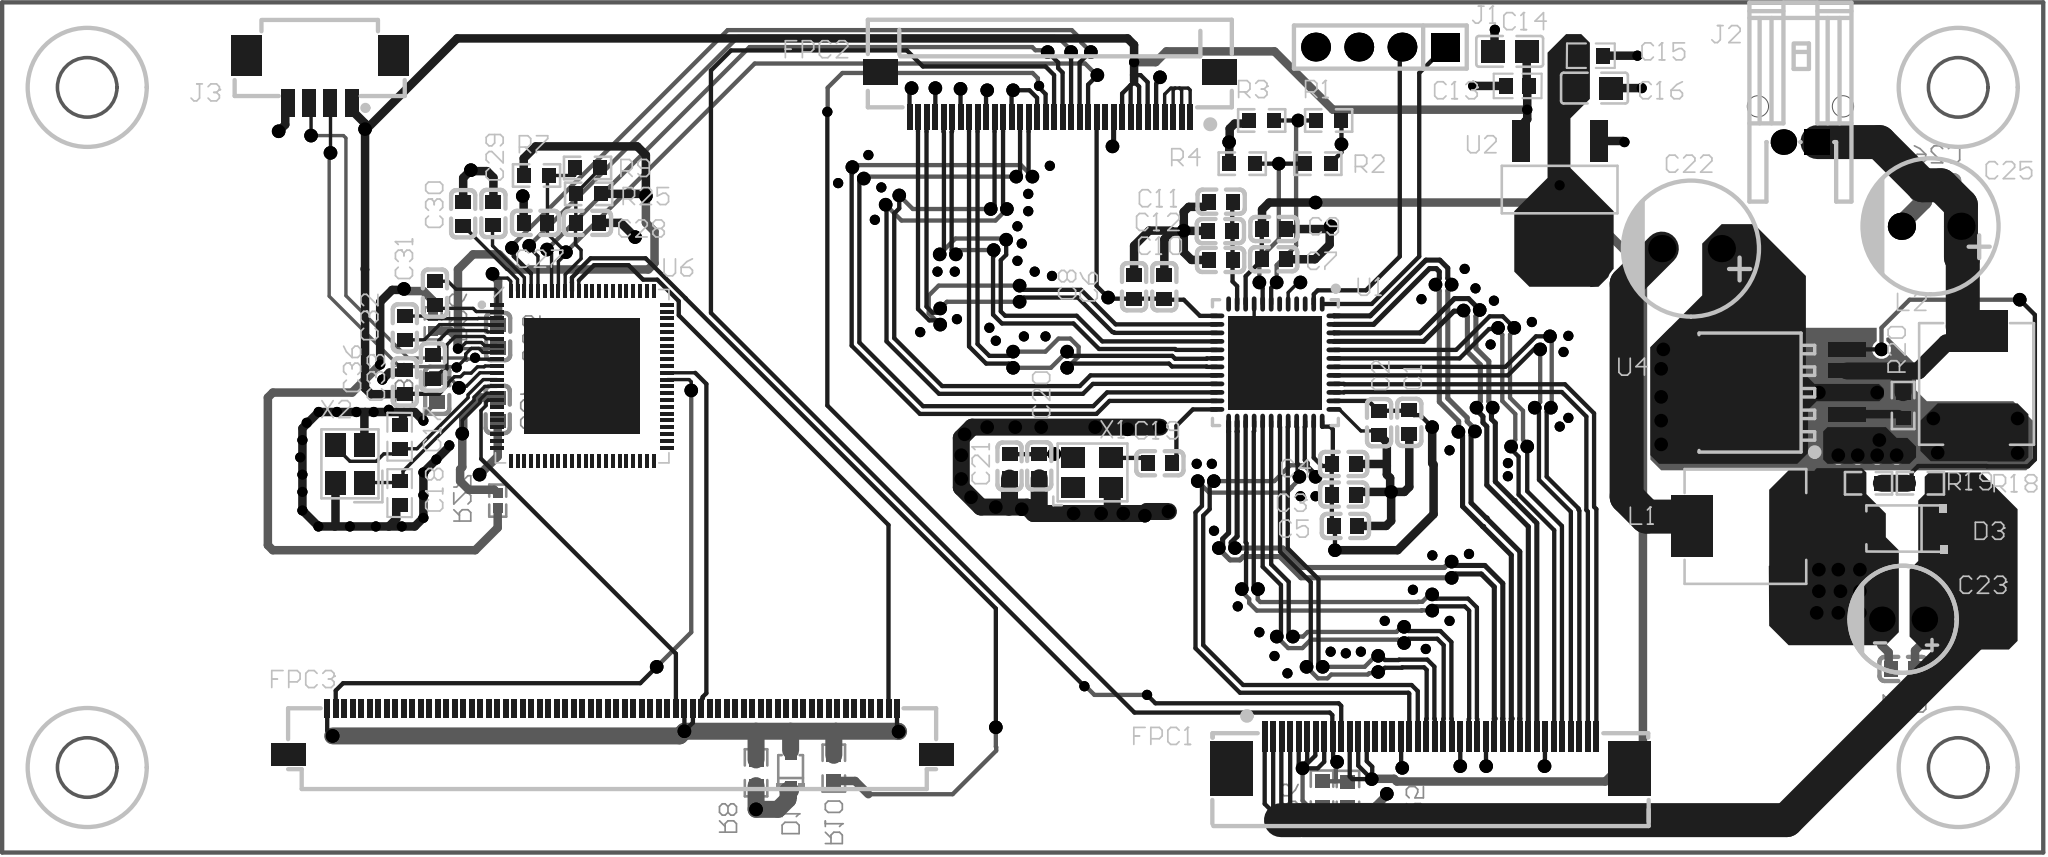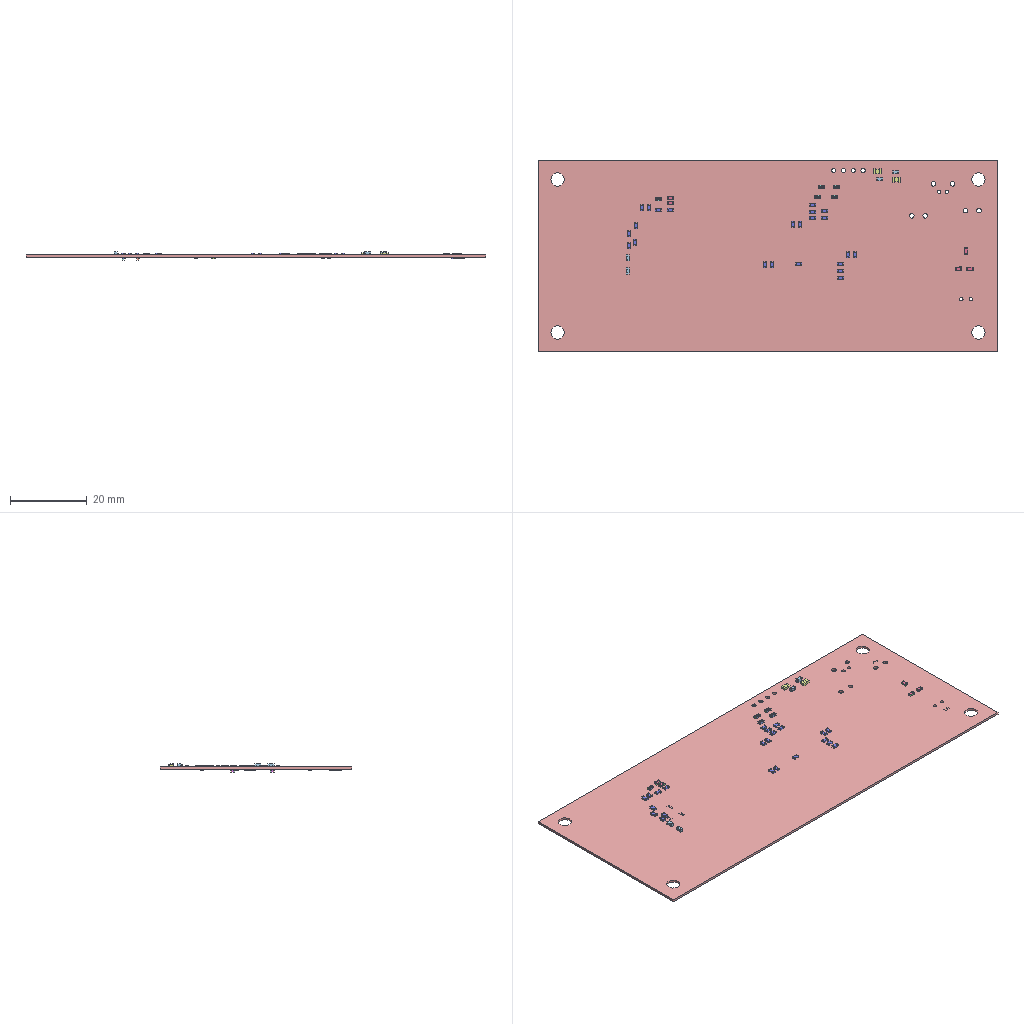Circuit board layout | Altium Designer | box 120 x 50 x 2.1 mm
Part placement:
Designator,Comment,Layer,Footprint,Center-X(mm),Center-Y(mm),Rotation
R10,0R 0603,BottomLayer,RES_R0603,48.895,4.962,270
R9,0R 5% NC,TopLayer,R0603,34.416,40.259,180
R8,0R 0603,BottomLayer,RES_R0603,44.323,4.69,90
X2,x322512msb4si,TopLayer,CRYSTAL-SMD_4P-L3.2-W2.5-BL,20.447,22.86,90
U2,bl1117-33cx,TopLayer,SOT-223_L6.5-W3.5-P2.30-LS7.0-BR,91.567,38.989,90
R7,10K 0603 1% NC,TopLayer,RES_R0603,31.417,39.818,180
D1,pdyl240b,BottomLayer,SOD-323_L1.8-W1.3-LS2.5-RD,46.355,4.827,90
C18,CC0603JRNPO9BN120,TopLayer,CAP_C0603,23.368,21.147,90
C17,CC0603JRNPO9BN120,TopLayer,CAP_C0603,23.368,24.446,270
C16,10uF 25V 0805,TopLayer,CAP_C0805,93.615,44.958,180
C15,100nF 50V 0603,TopLayer,CAP_C0603,93.41,46.863,0
C14,10uF 25V 0805,TopLayer,CAP_C0805,88.63,47.117,0
C13,100nF 50V 0603,TopLayer,CAP_C0603,89.089,45.085,180
R6,10K 0603 1%,BottomLayer,RES_R0603,77.597,3.438,270
R5,10K 0603 1%,BottomLayer,RES_R0603,79.121,3.42,90
R2,10K 0603 1%,TopLayer,RES_R0603,77.352,40.513,180
R4,10K 0603 1%,TopLayer,RES_R0603,72.907,40.513,180
R3,10K 0603 1%,TopLayer,RES_R0603,74.05,43.053,180
R1,10K 0603 1%,TopLayer,RES_R0603,77.987,43.053,180
J3,mx1.25mm-4p-wt,TopLayer,CONN-SMD_MX1.25MM-4P-WT,18.669,45.466,180
D3,ss34,TopLayer,SMA_L4.3-W2.6-LS5.0-RD,111.759,19.05,180
X1,ot322526mjba4sl,TopLayer,OSC-SMD_4P-L3.2-W2.5-BL,64.084,22.333,0
U6,ILI2511/QFN-88/10X10,TopLayer,ILI2511/QFN-88/10X10,34.101,28.015,0
U4,xl6008e1,TopLayer,TO-252-5_L6.6-W5.8-P1.27-TL,104.902,27.051,180
U1,GM8775C,TopLayer,UFQFPN-48_L7.0-W7.0-P0.50-BL-EP,74.857,28.811,180
R27,0R 5%,BottomLayer,R0402,29.134,20.695,90
R26,0R 5%,BottomLayer,R0402,25.342,31.121,270
R25,0R 5%,TopLayer,R0603,34.479,38.737,0
R20,rt0603brd0710kl,TopLayer,R0603,111.76,26.29,90
R19,rt0603brd0710kl,TopLayer,R0603,109.727,21.717,180
R18,rt0603brd0786k6l,TopLayer,R0603,112.777,21.717,0
L2,fxl0630-150-m,TopLayer,IND-SMD_L7.0-W6.6_FXL0630,116.078,27.559,270
L1,fxl0630-150-m,TopLayer,IND-SMD_L7.0-W6.6_FXL0630,102.489,19.177,180
J2,s02b-pask-2(lf)(sn),TopLayer,CONN-TH_S02B-PASK-2-LF-SN,105.724,41.783,0
J1,hx pz2.54-1x4p zz,TopLayer,HDR-TH_4P-P2.54-V-M,81.026,47.371,180
FPC3,afc18-s68fia-00,TopLayer,CONN-SMD_AFC18-S68FIA-00,35.86,7.134,0
FPC2,fc-05a34p011h20,TopLayer,FPC-SMD_FC-05A34P011H20,61.595,44.577,180
FPC1,fc-05d40p11h20,TopLayer,FPC-SMD_40P-P0.50_FC-05D40P11H20,83.976,5.875,0
C37,1u X7R 10% 6.3V,BottomLayer,C0603,29.136,26.059,90
C36,1u X7R 10% 6.3V,TopLayer,C0603,23.675,27.677,270
C35,1u X7R 10% 6.3V,BottomLayer,C0603,29.157,30.344,270
C34,1u X7R 10% 6.3V,BottomLayer,C0603,25.58,27.187,90
C33,1u X7R 10% 50V,TopLayer,C0603,25.326,28.551,270
C32,1u X7R 10% 50V,TopLayer,C0603,23.675,30.852,270
C31,1u X7R 10% 50V,TopLayer,C0603,25.446,32.899,270
C30,1u X7R 10% 50V,TopLayer,C0603,27.104,37.568,270
C29,1u X7R 10% 50V,TopLayer,C0603,28.882,37.583,270
C28,2.2u X7R 10% 6.3V,TopLayer,C0603,34.408,37.031,180
C27,0.1u X7R 10% 6.3V,TopLayer,C0603,31.36,37.031,180
C26,cc0603krx7r0bb104,BottomLayer,C0603,113.666,39.116,0
C25,era63v100m8x12,TopLayer,CAP-TH_BD8.0-P3.50-D0.8-FD,113.411,36.83,180
C24,cc0603krx7r0bb104,BottomLayer,C0603,111.761,10.795,0
C23,erg25v220m6x11,TopLayer,CAP-TH_BD6.3-P2.50-D0.5-FD,111.76,13.716,180
C22,era63v100m8x12,TopLayer,CAP-TH_BD8.0-P3.50-D0.8-FD,99.325,35.519,180
C21,cc0603krx7r0bb104,TopLayer,C0603,59.224,22.727,90
C20,cc0603krx7r0bb103,TopLayer,C0603,60.97,22.742,90
C19,cc0603krx7r9bb102,TopLayer,C0603,68.063,22.893,180
C12,cc0603krx7r8bb105,TopLayer,C0603,71.619,36.545,180
C11,cc0603krx7r0bb104,TopLayer,C0603,71.667,38.28,0
C10,cc0603krx7r0bb103,TopLayer,C0603,71.637,34.851,0
C9,cc0603krx7r0bb104,TopLayer,C0603,74.77,36.668,180
C8,cc0603krx7r0bb104,TopLayer,C0603,66.548,33.273,270
C7,cc0603krx7r0bb103,TopLayer,C0603,74.755,34.89,180
C6,cc0603krx7r0bb103,TopLayer,C0603,68.326,33.273,270
C5,cc0603krx7r8bb105,TopLayer,C0603,78.972,19.207,0
C4,cc0603krx7r0bb104,TopLayer,C0603,78.867,22.85,180
C3,cc0603krx7r0bb104,TopLayer,C0603,78.873,21.052,180
C2,cc0603krx7r0bb103,TopLayer,C0603,80.95,25.282,90
C1,cc0603krx7r0bb103,TopLayer,C0603,82.728,25.297,90